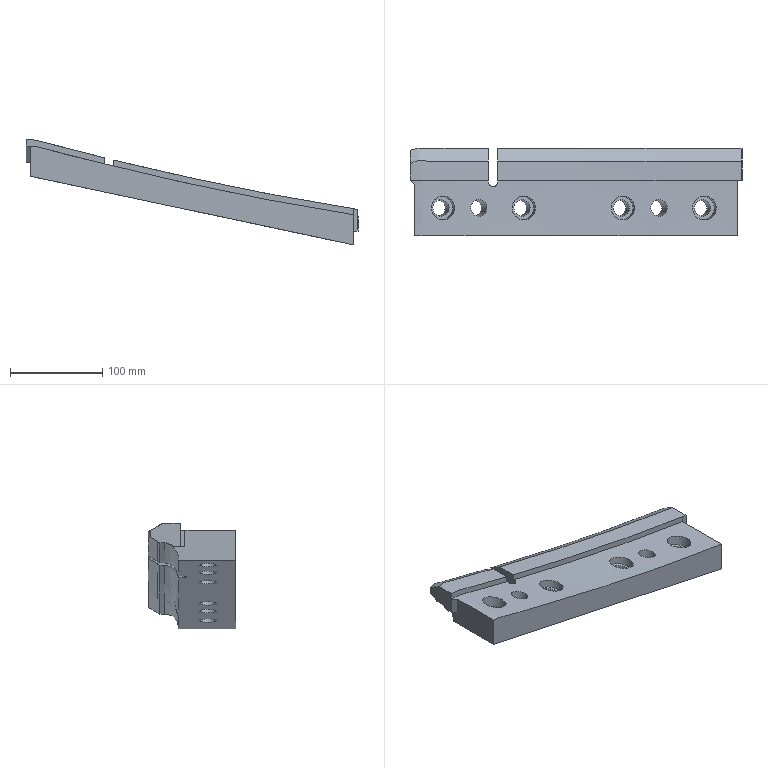Part | NX | features solid 2 | 1 solid | 44 faces | box 360 x 94.729 x 114.621 mm | volume 845415 mm3 | plane 18 | spline 15 | cylinder 11 | commonest cylinder face diameters 18 x6 26 x4 10 x1